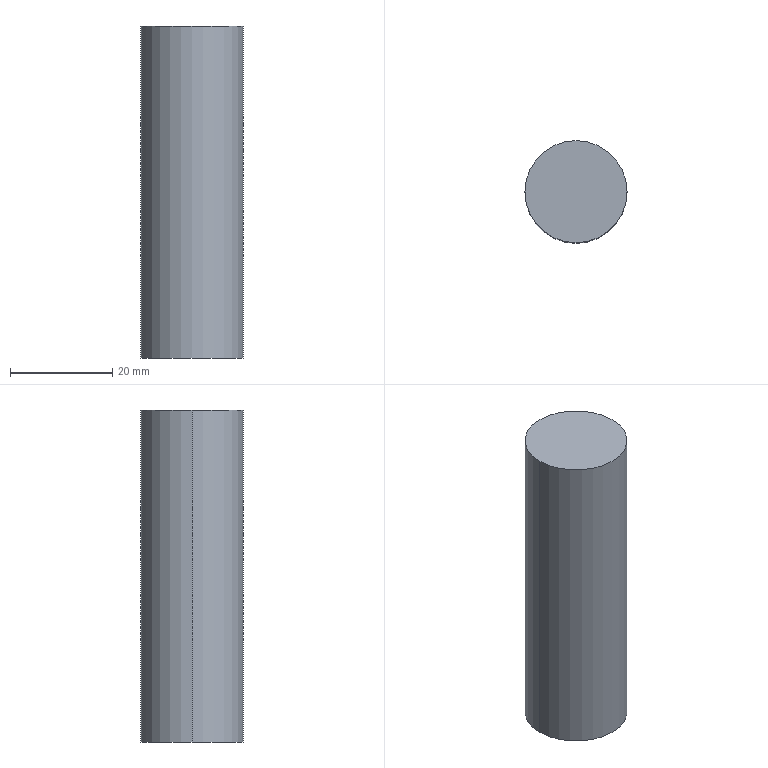Part | SolidWorks | features BaseBody 1 | 1 solid | 4 faces | box 20 x 20 x 65 mm | volume 20420 mm3 | plane 2 | cylinder 2 | commonest cylinder face diameters 20 x2
STEP:
#1=CARTESIAN_POINT('',(-10.,0.,0.));
#2=VERTEX_POINT('',#1);
#3=CARTESIAN_POINT('',(10.,0.,0.));
#4=VERTEX_POINT('',#3);
#5=CARTESIAN_POINT('',(0.,0.,0.));
#6=DIRECTION('',(0.,0.,1.));
#7=DIRECTION('',(1.,0.,0.));
#8=AXIS2_PLACEMENT_3D('',#5,#6,#7);
#9=CIRCLE('',#8,10.);
#10=EDGE_CURVE('',#2,#4,#9,.T.);
#11=ORIENTED_EDGE('',*,*,#10,.F.);
#12=CARTESIAN_POINT('',(0.,0.,0.));
#13=DIRECTION('',(0.,0.,1.));
#14=DIRECTION('',(1.,0.,0.));
#15=AXIS2_PLACEMENT_3D('',#12,#13,#14);
#16=CIRCLE('',#15,10.);
#17=EDGE_CURVE('',#4,#2,#16,.T.);
#18=ORIENTED_EDGE('',*,*,#17,.F.);
#19=EDGE_LOOP('',(#11,#18));
#20=FACE_OUTER_BOUND('',#19,.T.);
#21=CARTESIAN_POINT('',(0.,0.,0.));
#22=DIRECTION('',(0.,0.,1.));
#23=DIRECTION('',(1.,0.,0.));
#24=AXIS2_PLACEMENT_3D('',#21,#22,#23);
#25=PLANE('',#24);
#26=ADVANCED_FACE('',(#20),#25,.F.);
#27=CARTESIAN_POINT('',(-10.,0.,65.));
#28=VERTEX_POINT('',#27);
#29=CARTESIAN_POINT('',(10.,0.,65.));
#30=VERTEX_POINT('',#29);
#31=CARTESIAN_POINT('',(0.,0.,65.));
#32=DIRECTION('',(0.,0.,1.));
#33=DIRECTION('',(1.,0.,0.));
#34=AXIS2_PLACEMENT_3D('',#31,#32,#33);
#35=CIRCLE('',#34,10.);
#36=EDGE_CURVE('',#28,#30,#35,.T.);
#37=ORIENTED_EDGE('',*,*,#36,.T.);
#38=CARTESIAN_POINT('',(0.,0.,65.));
#39=DIRECTION('',(0.,0.,1.));
#40=DIRECTION('',(1.,0.,0.));
#41=AXIS2_PLACEMENT_3D('',#38,#39,#40);
#42=CIRCLE('',#41,10.);
#43=EDGE_CURVE('',#30,#28,#42,.T.);
#44=ORIENTED_EDGE('',*,*,#43,.T.);
#45=EDGE_LOOP('',(#37,#44));
#46=FACE_OUTER_BOUND('',#45,.T.);
#47=CARTESIAN_POINT('',(0.,0.,65.));
#48=DIRECTION('',(0.,0.,1.));
#49=DIRECTION('',(1.,0.,0.));
#50=AXIS2_PLACEMENT_3D('',#47,#48,#49);
#51=PLANE('',#50);
#52=ADVANCED_FACE('',(#46),#51,.T.);
#53=CARTESIAN_POINT('',(10.,0.,65.));
#54=DIRECTION('',(0.,0.,-1.));
#55=VECTOR('',#54,1000.);
#56=LINE('',#53,#55);
#57=EDGE_CURVE('',#30,#4,#56,.T.);
#58=ORIENTED_EDGE('',*,*,#57,.F.);
#59=ORIENTED_EDGE('',*,*,#36,.F.);
#60=CARTESIAN_POINT('',(-10.,0.,65.));
#61=DIRECTION('',(0.,0.,-1.));
#62=VECTOR('',#61,1000.);
#63=LINE('',#60,#62);
#64=EDGE_CURVE('',#28,#2,#63,.T.);
#65=ORIENTED_EDGE('',*,*,#64,.T.);
#66=ORIENTED_EDGE('',*,*,#10,.T.);
#67=EDGE_LOOP('',(#58,#59,#65,#66));
#68=FACE_OUTER_BOUND('',#67,.T.);
#69=CARTESIAN_POINT('',(0.,0.,65.));
#70=DIRECTION('',(0.,0.,-1.));
#71=DIRECTION('',(-1.,0.,0.));
#72=AXIS2_PLACEMENT_3D('',#69,#70,#71);
#73=CYLINDRICAL_SURFACE('',#72,10.);
#74=ADVANCED_FACE('',(#68),#73,.T.);
#75=ORIENTED_EDGE('',*,*,#43,.F.);
#76=ORIENTED_EDGE('',*,*,#57,.T.);
#77=ORIENTED_EDGE('',*,*,#17,.T.);
#78=ORIENTED_EDGE('',*,*,#64,.F.);
#79=EDGE_LOOP('',(#75,#76,#77,#78));
#80=FACE_OUTER_BOUND('',#79,.T.);
#81=CARTESIAN_POINT('',(0.,0.,65.));
#82=DIRECTION('',(0.,0.,-1.));
#83=DIRECTION('',(-1.,0.,0.));
#84=AXIS2_PLACEMENT_3D('',#81,#82,#83);
#85=CYLINDRICAL_SURFACE('',#84,10.);
#86=ADVANCED_FACE('',(#80),#85,.T.);
#87=CLOSED_SHELL('',(#26,#52,#74,#86));
#88=MANIFOLD_SOLID_BREP('',#87);
#89=CARTESIAN_POINT('',(0.,0.,0.));
#90=DIRECTION('',(0.,0.,1.));
#91=DIRECTION('',(1.,0.,0.));
#92=AXIS2_PLACEMENT_3D('',#89,#90,#91);
#93=(LENGTH_UNIT()NAMED_UNIT(*)SI_UNIT(.MILLI.,.METRE.));
#94=UNCERTAINTY_MEASURE_WITH_UNIT(LENGTH_MEASURE(0.00001),#93,'','');
#95=(NAMED_UNIT(*)PLANE_ANGLE_UNIT()SI_UNIT($,.RADIAN.));
#96=(NAMED_UNIT(*)SI_UNIT($,.STERADIAN.)SOLID_ANGLE_UNIT());
#97=(GEOMETRIC_REPRESENTATION_CONTEXT(3)GLOBAL_UNCERTAINTY_ASSIGNED_CONTEXT((#94))GLOBAL_UNIT_ASSIGNED_CONTEXT((#93,#95,#96))REPRESENTATION_CONTEXT('',''));
#98=ADVANCED_BREP_SHAPE_REPRESENTATION('',(#88,#92),#97);